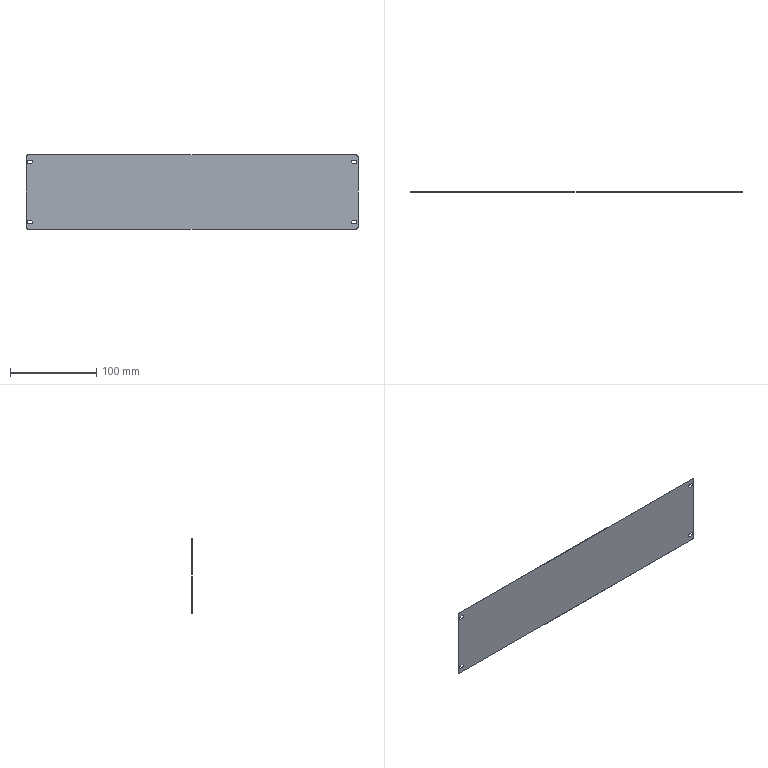Part | STEP file | LES120 steel strip^FTH120-PD-direct-drive motor | 1 solid | 26 faces | box 385.8 x 0.15 x 86 mm | volume 4964 mm3 | plane 14 | cylinder 12 | commonest cylinder face diameters 4 x12
STEP:
#1=CARTESIAN_POINT('',(190.9,0.15,-43.));
#2=VERTEX_POINT('',#1);
#3=CARTESIAN_POINT('',(192.9,0.15,-41.));
#4=VERTEX_POINT('',#3);
#5=CARTESIAN_POINT('',(190.9,0.15,-41.));
#6=DIRECTION('',(0.,-1.,0.));
#7=DIRECTION('',(0.,0.,-1.));
#8=AXIS2_PLACEMENT_3D('',#5,#6,#7);
#9=CIRCLE('',#8,2.);
#10=EDGE_CURVE('',#2,#4,#9,.T.);
#11=ORIENTED_EDGE('',*,*,#10,.F.);
#12=CARTESIAN_POINT('',(-190.9,0.15,-43.));
#13=VERTEX_POINT('',#12);
#14=CARTESIAN_POINT('',(0.,0.15,-43.));
#15=DIRECTION('',(1.,0.,0.));
#16=VECTOR('',#15,1000.);
#17=LINE('',#14,#16);
#18=EDGE_CURVE('',#13,#2,#17,.T.);
#19=ORIENTED_EDGE('',*,*,#18,.F.);
#20=CARTESIAN_POINT('',(-192.9,0.15,-41.));
#21=VERTEX_POINT('',#20);
#22=CARTESIAN_POINT('',(-190.9,0.15,-41.));
#23=DIRECTION('',(0.,-1.,0.));
#24=DIRECTION('',(0.,0.,-1.));
#25=AXIS2_PLACEMENT_3D('',#22,#23,#24);
#26=CIRCLE('',#25,2.);
#27=EDGE_CURVE('',#21,#13,#26,.T.);
#28=ORIENTED_EDGE('',*,*,#27,.F.);
#29=CARTESIAN_POINT('',(-192.9,0.15,41.));
#30=VERTEX_POINT('',#29);
#31=CARTESIAN_POINT('',(-192.9,0.15,0.));
#32=DIRECTION('',(0.,0.,-1.));
#33=VECTOR('',#32,1000.);
#34=LINE('',#31,#33);
#35=EDGE_CURVE('',#30,#21,#34,.T.);
#36=ORIENTED_EDGE('',*,*,#35,.F.);
#37=CARTESIAN_POINT('',(-190.9,0.15,43.));
#38=VERTEX_POINT('',#37);
#39=CARTESIAN_POINT('',(-190.9,0.15,41.));
#40=DIRECTION('',(0.,-1.,0.));
#41=DIRECTION('',(0.,0.,-1.));
#42=AXIS2_PLACEMENT_3D('',#39,#40,#41);
#43=CIRCLE('',#42,2.);
#44=EDGE_CURVE('',#38,#30,#43,.T.);
#45=ORIENTED_EDGE('',*,*,#44,.F.);
#46=CARTESIAN_POINT('',(190.9,0.15,43.));
#47=VERTEX_POINT('',#46);
#48=CARTESIAN_POINT('',(0.,0.15,43.));
#49=DIRECTION('',(-1.,0.,0.));
#50=VECTOR('',#49,1000.);
#51=LINE('',#48,#50);
#52=EDGE_CURVE('',#47,#38,#51,.T.);
#53=ORIENTED_EDGE('',*,*,#52,.F.);
#54=CARTESIAN_POINT('',(192.9,0.15,41.));
#55=VERTEX_POINT('',#54);
#56=CARTESIAN_POINT('',(190.9,0.15,41.));
#57=DIRECTION('',(0.,-1.,0.));
#58=DIRECTION('',(0.,0.,-1.));
#59=AXIS2_PLACEMENT_3D('',#56,#57,#58);
#60=CIRCLE('',#59,2.);
#61=EDGE_CURVE('',#55,#47,#60,.T.);
#62=ORIENTED_EDGE('',*,*,#61,.F.);
#63=CARTESIAN_POINT('',(192.9,0.15,0.));
#64=DIRECTION('',(0.,0.,1.));
#65=VECTOR('',#64,1000.);
#66=LINE('',#63,#65);
#67=EDGE_CURVE('',#4,#55,#66,.T.);
#68=ORIENTED_EDGE('',*,*,#67,.F.);
#69=EDGE_LOOP('',(#11,#19,#28,#36,#45,#53,#62,#68));
#70=FACE_OUTER_BOUND('',#69,.T.);
#71=CARTESIAN_POINT('',(-187.4,0.15,-32.9));
#72=VERTEX_POINT('',#71);
#73=CARTESIAN_POINT('',(-187.4,0.15,-36.9));
#74=VERTEX_POINT('',#73);
#75=CARTESIAN_POINT('',(-187.4,0.15,-34.9));
#76=DIRECTION('',(0.,1.,0.));
#77=DIRECTION('',(0.,0.,1.));
#78=AXIS2_PLACEMENT_3D('',#75,#76,#77);
#79=CIRCLE('',#78,2.);
#80=EDGE_CURVE('',#72,#74,#79,.T.);
#81=ORIENTED_EDGE('',*,*,#80,.F.);
#82=CARTESIAN_POINT('',(-189.4,0.15,-32.9));
#83=VERTEX_POINT('',#82);
#84=CARTESIAN_POINT('',(0.,0.15,-32.9));
#85=DIRECTION('',(1.,0.,0.));
#86=VECTOR('',#85,1000.);
#87=LINE('',#84,#86);
#88=EDGE_CURVE('',#83,#72,#87,.T.);
#89=ORIENTED_EDGE('',*,*,#88,.F.);
#90=CARTESIAN_POINT('',(-189.4,0.15,-36.9));
#91=VERTEX_POINT('',#90);
#92=CARTESIAN_POINT('',(-189.4,0.15,-34.9));
#93=DIRECTION('',(0.,1.,0.));
#94=DIRECTION('',(0.,0.,1.));
#95=AXIS2_PLACEMENT_3D('',#92,#93,#94);
#96=CIRCLE('',#95,2.);
#97=EDGE_CURVE('',#91,#83,#96,.T.);
#98=ORIENTED_EDGE('',*,*,#97,.F.);
#99=CARTESIAN_POINT('',(0.,0.15,-36.9));
#100=DIRECTION('',(-1.,0.,0.));
#101=VECTOR('',#100,1000.);
#102=LINE('',#99,#101);
#103=EDGE_CURVE('',#74,#91,#102,.T.);
#104=ORIENTED_EDGE('',*,*,#103,.F.);
#105=EDGE_LOOP('',(#81,#89,#98,#104));
#106=FACE_BOUND('',#105,.T.);
#107=CARTESIAN_POINT('',(-189.4,0.15,32.9));
#108=VERTEX_POINT('',#107);
#109=CARTESIAN_POINT('',(-189.4,0.15,36.9));
#110=VERTEX_POINT('',#109);
#111=CARTESIAN_POINT('',(-189.4,0.15,34.9));
#112=DIRECTION('',(0.,1.,0.));
#113=DIRECTION('',(0.,0.,1.));
#114=AXIS2_PLACEMENT_3D('',#111,#112,#113);
#115=CIRCLE('',#114,2.);
#116=EDGE_CURVE('',#108,#110,#115,.T.);
#117=ORIENTED_EDGE('',*,*,#116,.F.);
#118=CARTESIAN_POINT('',(-187.4,0.15,32.9));
#119=VERTEX_POINT('',#118);
#120=CARTESIAN_POINT('',(0.,0.15,32.9));
#121=DIRECTION('',(-1.,0.,0.));
#122=VECTOR('',#121,1000.);
#123=LINE('',#120,#122);
#124=EDGE_CURVE('',#119,#108,#123,.T.);
#125=ORIENTED_EDGE('',*,*,#124,.F.);
#126=CARTESIAN_POINT('',(-187.4,0.15,36.9));
#127=VERTEX_POINT('',#126);
#128=CARTESIAN_POINT('',(-187.4,0.15,34.9));
#129=DIRECTION('',(0.,1.,0.));
#130=DIRECTION('',(0.,0.,1.));
#131=AXIS2_PLACEMENT_3D('',#128,#129,#130);
#132=CIRCLE('',#131,2.);
#133=EDGE_CURVE('',#127,#119,#132,.T.);
#134=ORIENTED_EDGE('',*,*,#133,.F.);
#135=CARTESIAN_POINT('',(0.,0.15,36.9));
#136=DIRECTION('',(1.,0.,0.));
#137=VECTOR('',#136,1000.);
#138=LINE('',#135,#137);
#139=EDGE_CURVE('',#110,#127,#138,.T.);
#140=ORIENTED_EDGE('',*,*,#139,.F.);
#141=EDGE_LOOP('',(#117,#125,#134,#140));
#142=FACE_BOUND('',#141,.T.);
#143=CARTESIAN_POINT('',(189.4,0.15,36.9));
#144=VERTEX_POINT('',#143);
#145=CARTESIAN_POINT('',(189.4,0.15,32.9));
#146=VERTEX_POINT('',#145);
#147=CARTESIAN_POINT('',(189.4,0.15,34.9));
#148=DIRECTION('',(0.,1.,0.));
#149=DIRECTION('',(0.,0.,1.));
#150=AXIS2_PLACEMENT_3D('',#147,#148,#149);
#151=CIRCLE('',#150,2.);
#152=EDGE_CURVE('',#144,#146,#151,.T.);
#153=ORIENTED_EDGE('',*,*,#152,.F.);
#154=CARTESIAN_POINT('',(187.4,0.15,36.9));
#155=VERTEX_POINT('',#154);
#156=CARTESIAN_POINT('',(0.,0.15,36.9));
#157=DIRECTION('',(1.,0.,0.));
#158=VECTOR('',#157,1000.);
#159=LINE('',#156,#158);
#160=EDGE_CURVE('',#155,#144,#159,.T.);
#161=ORIENTED_EDGE('',*,*,#160,.F.);
#162=CARTESIAN_POINT('',(187.4,0.15,32.9));
#163=VERTEX_POINT('',#162);
#164=CARTESIAN_POINT('',(187.4,0.15,34.9));
#165=DIRECTION('',(0.,1.,0.));
#166=DIRECTION('',(0.,0.,1.));
#167=AXIS2_PLACEMENT_3D('',#164,#165,#166);
#168=CIRCLE('',#167,2.);
#169=EDGE_CURVE('',#163,#155,#168,.T.);
#170=ORIENTED_EDGE('',*,*,#169,.F.);
#171=CARTESIAN_POINT('',(0.,0.15,32.9));
#172=DIRECTION('',(-1.,0.,0.));
#173=VECTOR('',#172,1000.);
#174=LINE('',#171,#173);
#175=EDGE_CURVE('',#146,#163,#174,.T.);
#176=ORIENTED_EDGE('',*,*,#175,.F.);
#177=EDGE_LOOP('',(#153,#161,#170,#176));
#178=FACE_BOUND('',#177,.T.);
#179=CARTESIAN_POINT('',(189.4,0.15,-32.9));
#180=VERTEX_POINT('',#179);
#181=CARTESIAN_POINT('',(189.4,0.15,-36.9));
#182=VERTEX_POINT('',#181);
#183=CARTESIAN_POINT('',(189.4,0.15,-34.9));
#184=DIRECTION('',(0.,1.,0.));
#185=DIRECTION('',(0.,0.,1.));
#186=AXIS2_PLACEMENT_3D('',#183,#184,#185);
#187=CIRCLE('',#186,2.);
#188=EDGE_CURVE('',#180,#182,#187,.T.);
#189=ORIENTED_EDGE('',*,*,#188,.F.);
#190=CARTESIAN_POINT('',(187.4,0.15,-32.9));
#191=VERTEX_POINT('',#190);
#192=CARTESIAN_POINT('',(0.,0.15,-32.9));
#193=DIRECTION('',(1.,0.,0.));
#194=VECTOR('',#193,1000.);
#195=LINE('',#192,#194);
#196=EDGE_CURVE('',#191,#180,#195,.T.);
#197=ORIENTED_EDGE('',*,*,#196,.F.);
#198=CARTESIAN_POINT('',(187.4,0.15,-36.9));
#199=VERTEX_POINT('',#198);
#200=CARTESIAN_POINT('',(187.4,0.15,-34.9));
#201=DIRECTION('',(0.,1.,0.));
#202=DIRECTION('',(0.,0.,1.));
#203=AXIS2_PLACEMENT_3D('',#200,#201,#202);
#204=CIRCLE('',#203,2.);
#205=EDGE_CURVE('',#199,#191,#204,.T.);
#206=ORIENTED_EDGE('',*,*,#205,.F.);
#207=CARTESIAN_POINT('',(0.,0.15,-36.9));
#208=DIRECTION('',(-1.,0.,0.));
#209=VECTOR('',#208,1000.);
#210=LINE('',#207,#209);
#211=EDGE_CURVE('',#182,#199,#210,.T.);
#212=ORIENTED_EDGE('',*,*,#211,.F.);
#213=EDGE_LOOP('',(#189,#197,#206,#212));
#214=FACE_BOUND('',#213,.T.);
#215=CARTESIAN_POINT('',(0.,0.15,0.));
#216=DIRECTION('',(0.,-1.,0.));
#217=DIRECTION('',(0.,0.,-1.));
#218=AXIS2_PLACEMENT_3D('',#215,#216,#217);
#219=PLANE('',#218);
#220=ADVANCED_FACE('',(#70,#106,#142,#178,#214),#219,.F.);
#221=CARTESIAN_POINT('',(192.9,0.,-41.));
#222=VERTEX_POINT('',#221);
#223=CARTESIAN_POINT('',(192.9,0.15,-41.));
#224=DIRECTION('',(0.,-1.,0.));
#225=VECTOR('',#224,1000.);
#226=LINE('',#223,#225);
#227=EDGE_CURVE('',#4,#222,#226,.T.);
#228=ORIENTED_EDGE('',*,*,#227,.F.);
#229=ORIENTED_EDGE('',*,*,#67,.T.);
#230=CARTESIAN_POINT('',(192.9,0.,41.));
#231=VERTEX_POINT('',#230);
#232=CARTESIAN_POINT('',(192.9,0.15,41.));
#233=DIRECTION('',(0.,1.,0.));
#234=VECTOR('',#233,1000.);
#235=LINE('',#232,#234);
#236=EDGE_CURVE('',#231,#55,#235,.T.);
#237=ORIENTED_EDGE('',*,*,#236,.F.);
#238=CARTESIAN_POINT('',(192.9,0.,43.));
#239=DIRECTION('',(0.,0.,1.));
#240=VECTOR('',#239,1000.);
#241=LINE('',#238,#240);
#242=EDGE_CURVE('',#222,#231,#241,.T.);
#243=ORIENTED_EDGE('',*,*,#242,.F.);
#244=EDGE_LOOP('',(#228,#229,#237,#243));
#245=FACE_OUTER_BOUND('',#244,.T.);
#246=CARTESIAN_POINT('',(192.9,0.15,43.));
#247=DIRECTION('',(-1.,0.,0.));
#248=DIRECTION('',(0.,0.,1.));
#249=AXIS2_PLACEMENT_3D('',#246,#247,#248);
#250=PLANE('',#249);
#251=ADVANCED_FACE('',(#245),#250,.F.);
#252=CARTESIAN_POINT('',(190.9,0.,-43.));
#253=VERTEX_POINT('',#252);
#254=CARTESIAN_POINT('',(190.9,0.,-41.));
#255=DIRECTION('',(0.,1.,0.));
#256=DIRECTION('',(0.,0.,-1.));
#257=AXIS2_PLACEMENT_3D('',#254,#255,#256);
#258=CIRCLE('',#257,2.);
#259=EDGE_CURVE('',#222,#253,#258,.T.);
#260=ORIENTED_EDGE('',*,*,#259,.T.);
#261=CARTESIAN_POINT('',(190.9,0.15,-43.));
#262=DIRECTION('',(0.,1.,0.));
#263=VECTOR('',#262,1000.);
#264=LINE('',#261,#263);
#265=EDGE_CURVE('',#253,#2,#264,.T.);
#266=ORIENTED_EDGE('',*,*,#265,.T.);
#267=ORIENTED_EDGE('',*,*,#10,.T.);
#268=ORIENTED_EDGE('',*,*,#227,.T.);
#269=EDGE_LOOP('',(#260,#266,#267,#268));
#270=FACE_OUTER_BOUND('',#269,.T.);
#271=CARTESIAN_POINT('',(190.9,0.15,-41.));
#272=DIRECTION('',(0.,-1.,0.));
#273=DIRECTION('',(0.,0.,-1.));
#274=AXIS2_PLACEMENT_3D('',#271,#272,#273);
#275=CYLINDRICAL_SURFACE('',#274,2.);
#276=ADVANCED_FACE('',(#270),#275,.T.);
#277=ORIENTED_EDGE('',*,*,#265,.F.);
#278=CARTESIAN_POINT('',(-190.9,0.,-43.));
#279=VERTEX_POINT('',#278);
#280=CARTESIAN_POINT('',(-192.9,0.,-43.));
#281=DIRECTION('',(1.,0.,0.));
#282=VECTOR('',#281,1000.);
#283=LINE('',#280,#282);
#284=EDGE_CURVE('',#279,#253,#283,.T.);
#285=ORIENTED_EDGE('',*,*,#284,.F.);
#286=CARTESIAN_POINT('',(-190.9,0.15,-43.));
#287=DIRECTION('',(0.,-1.,0.));
#288=VECTOR('',#287,1000.);
#289=LINE('',#286,#288);
#290=EDGE_CURVE('',#13,#279,#289,.T.);
#291=ORIENTED_EDGE('',*,*,#290,.F.);
#292=ORIENTED_EDGE('',*,*,#18,.T.);
#293=EDGE_LOOP('',(#277,#285,#291,#292));
#294=FACE_OUTER_BOUND('',#293,.T.);
#295=CARTESIAN_POINT('',(-192.9,0.15,-43.));
#296=DIRECTION('',(0.,0.,1.));
#297=DIRECTION('',(1.,0.,0.));
#298=AXIS2_PLACEMENT_3D('',#295,#296,#297);
#299=PLANE('',#298);
#300=ADVANCED_FACE('',(#294),#299,.F.);
#301=CARTESIAN_POINT('',(-192.9,0.,-41.));
#302=VERTEX_POINT('',#301);
#303=CARTESIAN_POINT('',(-190.9,0.,-41.));
#304=DIRECTION('',(0.,1.,0.));
#305=DIRECTION('',(0.,0.,-1.));
#306=AXIS2_PLACEMENT_3D('',#303,#304,#305);
#307=CIRCLE('',#306,2.);
#308=EDGE_CURVE('',#279,#302,#307,.T.);
#309=ORIENTED_EDGE('',*,*,#308,.T.);
#310=CARTESIAN_POINT('',(-192.9,0.15,-41.));
#311=DIRECTION('',(0.,1.,0.));
#312=VECTOR('',#311,1000.);
#313=LINE('',#310,#312);
#314=EDGE_CURVE('',#302,#21,#313,.T.);
#315=ORIENTED_EDGE('',*,*,#314,.T.);
#316=ORIENTED_EDGE('',*,*,#27,.T.);
#317=ORIENTED_EDGE('',*,*,#290,.T.);
#318=EDGE_LOOP('',(#309,#315,#316,#317));
#319=FACE_OUTER_BOUND('',#318,.T.);
#320=CARTESIAN_POINT('',(-190.9,0.15,-41.));
#321=DIRECTION('',(0.,-1.,0.));
#322=DIRECTION('',(0.,0.,-1.));
#323=AXIS2_PLACEMENT_3D('',#320,#321,#322);
#324=CYLINDRICAL_SURFACE('',#323,2.);
#325=ADVANCED_FACE('',(#319),#324,.T.);
#326=ORIENTED_EDGE('',*,*,#314,.F.);
#327=CARTESIAN_POINT('',(-192.9,0.,41.));
#328=VERTEX_POINT('',#327);
#329=CARTESIAN_POINT('',(-192.9,0.,43.));
#330=DIRECTION('',(0.,0.,-1.));
#331=VECTOR('',#330,1000.);
#332=LINE('',#329,#331);
#333=EDGE_CURVE('',#328,#302,#332,.T.);
#334=ORIENTED_EDGE('',*,*,#333,.F.);
#335=CARTESIAN_POINT('',(-192.9,0.15,41.));
#336=DIRECTION('',(0.,-1.,0.));
#337=VECTOR('',#336,1000.);
#338=LINE('',#335,#337);
#339=EDGE_CURVE('',#30,#328,#338,.T.);
#340=ORIENTED_EDGE('',*,*,#339,.F.);
#341=ORIENTED_EDGE('',*,*,#35,.T.);
#342=EDGE_LOOP('',(#326,#334,#340,#341));
#343=FACE_OUTER_BOUND('',#342,.T.);
#344=CARTESIAN_POINT('',(-192.9,0.15,43.));
#345=DIRECTION('',(1.,0.,0.));
#346=DIRECTION('',(0.,0.,-1.));
#347=AXIS2_PLACEMENT_3D('',#344,#345,#346);
#348=PLANE('',#347);
#349=ADVANCED_FACE('',(#343),#348,.F.);
#350=CARTESIAN_POINT('',(-190.9,0.,43.));
#351=VERTEX_POINT('',#350);
#352=CARTESIAN_POINT('',(-190.9,0.,41.));
#353=DIRECTION('',(0.,1.,0.));
#354=DIRECTION('',(0.,0.,-1.));
#355=AXIS2_PLACEMENT_3D('',#352,#353,#354);
#356=CIRCLE('',#355,2.);
#357=EDGE_CURVE('',#328,#351,#356,.T.);
#358=ORIENTED_EDGE('',*,*,#357,.T.);
#359=CARTESIAN_POINT('',(-190.9,0.15,43.));
#360=DIRECTION('',(0.,1.,0.));
#361=VECTOR('',#360,1000.);
#362=LINE('',#359,#361);
#363=EDGE_CURVE('',#351,#38,#362,.T.);
#364=ORIENTED_EDGE('',*,*,#363,.T.);
#365=ORIENTED_EDGE('',*,*,#44,.T.);
#366=ORIENTED_EDGE('',*,*,#339,.T.);
#367=EDGE_LOOP('',(#358,#364,#365,#366));
#368=FACE_OUTER_BOUND('',#367,.T.);
#369=CARTESIAN_POINT('',(-190.9,0.15,41.));
#370=DIRECTION('',(0.,-1.,0.));
#371=DIRECTION('',(0.,0.,-1.));
#372=AXIS2_PLACEMENT_3D('',#369,#370,#371);
#373=CYLINDRICAL_SURFACE('',#372,2.);
#374=ADVANCED_FACE('',(#368),#373,.T.);
#375=CARTESIAN_POINT('',(190.9,0.,43.));
#376=VERTEX_POINT('',#375);
#377=CARTESIAN_POINT('',(190.9,0.15,43.));
#378=DIRECTION('',(0.,-1.,0.));
#379=VECTOR('',#378,1000.);
#380=LINE('',#377,#379);
#381=EDGE_CURVE('',#47,#376,#380,.T.);
#382=ORIENTED_EDGE('',*,*,#381,.F.);
#383=ORIENTED_EDGE('',*,*,#52,.T.);
#384=ORIENTED_EDGE('',*,*,#363,.F.);
#385=CARTESIAN_POINT('',(-192.9,0.,43.));
#386=DIRECTION('',(-1.,0.,0.));
#387=VECTOR('',#386,1000.);
#388=LINE('',#385,#387);
#389=EDGE_CURVE('',#376,#351,#388,.T.);
#390=ORIENTED_EDGE('',*,*,#389,.F.);
#391=EDGE_LOOP('',(#382,#383,#384,#390));
#392=FACE_OUTER_BOUND('',#391,.T.);
#393=CARTESIAN_POINT('',(-192.9,0.15,43.));
#394=DIRECTION('',(0.,0.,-1.));
#395=DIRECTION('',(-1.,0.,0.));
#396=AXIS2_PLACEMENT_3D('',#393,#394,#395);
#397=PLANE('',#396);
#398=ADVANCED_FACE('',(#392),#397,.F.);
#399=CARTESIAN_POINT('',(190.9,0.,41.));
#400=DIRECTION('',(0.,1.,0.));
#401=DIRECTION('',(0.,0.,-1.));
#402=AXIS2_PLACEMENT_3D('',#399,#400,#401);
#403=CIRCLE('',#402,2.);
#404=EDGE_CURVE('',#376,#231,#403,.T.);
#405=ORIENTED_EDGE('',*,*,#404,.T.);
#406=ORIENTED_EDGE('',*,*,#236,.T.);
#407=ORIENTED_EDGE('',*,*,#61,.T.);
#408=ORIENTED_EDGE('',*,*,#381,.T.);
#409=EDGE_LOOP('',(#405,#406,#407,#408));
#410=FACE_OUTER_BOUND('',#409,.T.);
#411=CARTESIAN_POINT('',(190.9,0.15,41.));
#412=DIRECTION('',(0.,-1.,0.));
#413=DIRECTION('',(0.,0.,-1.));
#414=AXIS2_PLACEMENT_3D('',#411,#412,#413);
#415=CYLINDRICAL_SURFACE('',#414,2.);
#416=ADVANCED_FACE('',(#410),#415,.T.);
#417=CARTESIAN_POINT('',(-189.4,0.,-36.9));
#418=VERTEX_POINT('',#417);
#419=CARTESIAN_POINT('',(-189.4,0.,-36.9));
#420=DIRECTION('',(0.,1.,0.));
#421=VECTOR('',#420,1000.);
#422=LINE('',#419,#421);
#423=EDGE_CURVE('',#418,#91,#422,.T.);
#424=ORIENTED_EDGE('',*,*,#423,.F.);
#425=CARTESIAN_POINT('',(-187.4,0.,-36.9));
#426=VERTEX_POINT('',#425);
#427=CARTESIAN_POINT('',(-189.4,0.,-36.9));
#428=DIRECTION('',(-1.,0.,0.));
#429=VECTOR('',#428,1000.);
#430=LINE('',#427,#429);
#431=EDGE_CURVE('',#426,#418,#430,.T.);
#432=ORIENTED_EDGE('',*,*,#431,.F.);
#433=CARTESIAN_POINT('',(-187.4,0.,-36.9));
#434=DIRECTION('',(0.,-1.,0.));
#435=VECTOR('',#434,1000.);
#436=LINE('',#433,#435);
#437=EDGE_CURVE('',#74,#426,#436,.T.);
#438=ORIENTED_EDGE('',*,*,#437,.F.);
#439=ORIENTED_EDGE('',*,*,#103,.T.);
#440=EDGE_LOOP('',(#424,#432,#438,#439));
#441=FACE_OUTER_BOUND('',#440,.T.);
#442=CARTESIAN_POINT('',(-189.4,0.,-36.9));
#443=DIRECTION('',(0.,0.,-1.));
#444=DIRECTION('',(-1.,0.,0.));
#445=AXIS2_PLACEMENT_3D('',#442,#443,#444);
#446=PLANE('',#445);
#447=ADVANCED_FACE('',(#441),#446,.F.);
#448=ORIENTED_EDGE('',*,*,#437,.T.);
#449=CARTESIAN_POINT('',(-187.4,0.,-32.9));
#450=VERTEX_POINT('',#449);
#451=CARTESIAN_POINT('',(-187.4,0.,-34.9));
#452=DIRECTION('',(0.,1.,0.));
#453=DIRECTION('',(0.,0.,1.));
#454=AXIS2_PLACEMENT_3D('',#451,#452,#453);
#455=CIRCLE('',#454,2.);
#456=EDGE_CURVE('',#450,#426,#455,.T.);
#457=ORIENTED_EDGE('',*,*,#456,.F.);
#458=CARTESIAN_POINT('',(-187.4,0.,-32.9));
#459=DIRECTION('',(0.,-1.,0.));
#460=VECTOR('',#459,1000.);
#461=LINE('',#458,#460);
#462=EDGE_CURVE('',#72,#450,#461,.T.);
#463=ORIENTED_EDGE('',*,*,#462,.F.);
#464=ORIENTED_EDGE('',*,*,#80,.T.);
#465=EDGE_LOOP('',(#448,#457,#463,#464));
#466=FACE_OUTER_BOUND('',#465,.T.);
#467=CARTESIAN_POINT('',(-187.4,0.,-34.9));
#468=DIRECTION('',(0.,1.,0.));
#469=DIRECTION('',(0.,0.,1.));
#470=AXIS2_PLACEMENT_3D('',#467,#468,#469);
#471=CYLINDRICAL_SURFACE('',#470,2.);
#472=ADVANCED_FACE('',(#466),#471,.F.);
#473=ORIENTED_EDGE('',*,*,#462,.T.);
#474=CARTESIAN_POINT('',(-189.4,0.,-32.9));
#475=VERTEX_POINT('',#474);
#476=CARTESIAN_POINT('',(-189.4,0.,-32.9));
#477=DIRECTION('',(1.,0.,0.));
#478=VECTOR('',#477,1000.);
#479=LINE('',#476,#478);
#480=EDGE_CURVE('',#475,#450,#479,.T.);
#481=ORIENTED_EDGE('',*,*,#480,.F.);
#482=CARTESIAN_POINT('',(-189.4,0.,-32.9));
#483=DIRECTION('',(0.,-1.,0.));
#484=VECTOR('',#483,1000.);
#485=LINE('',#482,#484);
#486=EDGE_CURVE('',#83,#475,#485,.T.);
#487=ORIENTED_EDGE('',*,*,#486,.F.);
#488=ORIENTED_EDGE('',*,*,#88,.T.);
#489=EDGE_LOOP('',(#473,#481,#487,#488));
#490=FACE_OUTER_BOUND('',#489,.T.);
#491=CARTESIAN_POINT('',(-189.4,0.,-32.9));
#492=DIRECTION('',(0.,0.,1.));
#493=DIRECTION('',(1.,0.,0.));
#494=AXIS2_PLACEMENT_3D('',#491,#492,#493);
#495=PLANE('',#494);
#496=ADVANCED_FACE('',(#490),#495,.F.);
#497=ORIENTED_EDGE('',*,*,#486,.T.);
#498=CARTESIAN_POINT('',(-189.4,0.,-34.9));
#499=DIRECTION('',(0.,1.,0.));
#500=DIRECTION('',(0.,0.,1.));
#501=AXIS2_PLACEMENT_3D('',#498,#499,#500);
#502=CIRCLE('',#501,2.);
#503=EDGE_CURVE('',#418,#475,#502,.T.);
#504=ORIENTED_EDGE('',*,*,#503,.F.);
#505=ORIENTED_EDGE('',*,*,#423,.T.);
#506=ORIENTED_EDGE('',*,*,#97,.T.);
#507=EDGE_LOOP('',(#497,#504,#505,#506));
#508=FACE_OUTER_BOUND('',#507,.T.);
#509=CARTESIAN_POINT('',(-189.4,0.,-34.9));
#510=DIRECTION('',(0.,1.,0.));
#511=DIRECTION('',(0.,0.,1.));
#512=AXIS2_PLACEMENT_3D('',#509,#510,#511);
#513=CYLINDRICAL_SURFACE('',#512,2.);
#514=ADVANCED_FACE('',(#508),#513,.F.);
#515=CARTESIAN_POINT('',(-187.4,0.,36.9));
#516=VERTEX_POINT('',#515);
#517=CARTESIAN_POINT('',(-187.4,0.,36.9));
#518=DIRECTION('',(0.,1.,0.));
#519=VECTOR('',#518,1000.);
#520=LINE('',#517,#519);
#521=EDGE_CURVE('',#516,#127,#520,.T.);
#522=ORIENTED_EDGE('',*,*,#521,.F.);
#523=CARTESIAN_POINT('',(-189.4,0.,36.9));
#524=VERTEX_POINT('',#523);
#525=CARTESIAN_POINT('',(-189.4,0.,36.9));
#526=DIRECTION('',(1.,0.,0.));
#527=VECTOR('',#526,1000.);
#528=LINE('',#525,#527);
#529=EDGE_CURVE('',#524,#516,#528,.T.);
#530=ORIENTED_EDGE('',*,*,#529,.F.);
#531=CARTESIAN_POINT('',(-189.4,0.,36.9));
#532=DIRECTION('',(0.,-1.,0.));
#533=VECTOR('',#532,1000.);
#534=LINE('',#531,#533);
#535=EDGE_CURVE('',#110,#524,#534,.T.);
#536=ORIENTED_EDGE('',*,*,#535,.F.);
#537=ORIENTED_EDGE('',*,*,#139,.T.);
#538=EDGE_LOOP('',(#522,#530,#536,#537));
#539=FACE_OUTER_BOUND('',#538,.T.);
#540=CARTESIAN_POINT('',(-189.4,0.,36.9));
#541=DIRECTION('',(0.,0.,1.));
#542=DIRECTION('',(1.,0.,0.));
#543=AXIS2_PLACEMENT_3D('',#540,#541,#542);
#544=PLANE('',#543);
#545=ADVANCED_FACE('',(#539),#544,.F.);
#546=ORIENTED_EDGE('',*,*,#535,.T.);
#547=CARTESIAN_POINT('',(-189.4,0.,32.9));
#548=VERTEX_POINT('',#547);
#549=CARTESIAN_POINT('',(-189.4,0.,34.9));
#550=DIRECTION('',(0.,1.,0.));
#551=DIRECTION('',(0.,0.,1.));
#552=AXIS2_PLACEMENT_3D('',#549,#550,#551);
#553=CIRCLE('',#552,2.);
#554=EDGE_CURVE('',#548,#524,#553,.T.);
#555=ORIENTED_EDGE('',*,*,#554,.F.);
#556=CARTESIAN_POINT('',(-189.4,0.,32.9));
#557=DIRECTION('',(0.,-1.,0.));
#558=VECTOR('',#557,1000.);
#559=LINE('',#556,#558);
#560=EDGE_CURVE('',#108,#548,#559,.T.);
#561=ORIENTED_EDGE('',*,*,#560,.F.);
#562=ORIENTED_EDGE('',*,*,#116,.T.);
#563=EDGE_LOOP('',(#546,#555,#561,#562));
#564=FACE_OUTER_BOUND('',#563,.T.);
#565=CARTESIAN_POINT('',(-189.4,0.,34.9));
#566=DIRECTION('',(0.,1.,0.));
#567=DIRECTION('',(0.,0.,1.));
#568=AXIS2_PLACEMENT_3D('',#565,#566,#567);
#569=CYLINDRICAL_SURFACE('',#568,2.);
#570=ADVANCED_FACE('',(#564),#569,.F.);
#571=ORIENTED_EDGE('',*,*,#560,.T.);
#572=CARTESIAN_POINT('',(-187.4,0.,32.9));
#573=VERTEX_POINT('',#572);
#574=CARTESIAN_POINT('',(-189.4,0.,32.9));
#575=DIRECTION('',(-1.,0.,0.));
#576=VECTOR('',#575,1000.);
#577=LINE('',#574,#576);
#578=EDGE_CURVE('',#573,#548,#577,.T.);
#579=ORIENTED_EDGE('',*,*,#578,.F.);
#580=CARTESIAN_POINT('',(-187.4,0.,32.9));
#581=DIRECTION('',(0.,-1.,0.));
#582=VECTOR('',#581,1000.);
#583=LINE('',#580,#582);
#584=EDGE_CURVE('',#119,#573,#583,.T.);
#585=ORIENTED_EDGE('',*,*,#584,.F.);
#586=ORIENTED_EDGE('',*,*,#124,.T.);
#587=EDGE_LOOP('',(#571,#579,#585,#586));
#588=FACE_OUTER_BOUND('',#587,.T.);
#589=CARTESIAN_POINT('',(-189.4,0.,32.9));
#590=DIRECTION('',(0.,0.,-1.));
#591=DIRECTION('',(-1.,0.,0.));
#592=AXIS2_PLACEMENT_3D('',#589,#590,#591);
#593=PLANE('',#592);
#594=ADVANCED_FACE('',(#588),#593,.F.);
#595=ORIENTED_EDGE('',*,*,#584,.T.);
#596=CARTESIAN_POINT('',(-187.4,0.,34.9));
#597=DIRECTION('',(0.,1.,0.));
#598=DIRECTION('',(0.,0.,1.));
#599=AXIS2_PLACEMENT_3D('',#596,#597,#598);
#600=CIRCLE('',#599,2.);
#601=EDGE_CURVE('',#516,#573,#600,.T.);
#602=ORIENTED_EDGE('',*,*,#601,.F.);
#603=ORIENTED_EDGE('',*,*,#521,.T.);
#604=ORIENTED_EDGE('',*,*,#133,.T.);
#605=EDGE_LOOP('',(#595,#602,#603,#604));
#606=FACE_OUTER_BOUND('',#605,.T.);
#607=CARTESIAN_POINT('',(-187.4,0.,34.9));
#608=DIRECTION('',(0.,1.,0.));
#609=DIRECTION('',(0.,0.,1.));
#610=AXIS2_PLACEMENT_3D('',#607,#608,#609);
#611=CYLINDRICAL_SURFACE('',#610,2.);
#612=ADVANCED_FACE('',(#606),#611,.F.);
#613=CARTESIAN_POINT('',(187.4,0.,32.9));
#614=VERTEX_POINT('',#613);
#615=CARTESIAN_POINT('',(187.4,0.,32.9));
#616=DIRECTION('',(0.,1.,0.));
#617=VECTOR('',#616,1000.);
#618=LINE('',#615,#617);
#619=EDGE_CURVE('',#614,#163,#618,.T.);
#620=ORIENTED_EDGE('',*,*,#619,.F.);
#621=CARTESIAN_POINT('',(189.4,0.,32.9));
#622=VERTEX_POINT('',#621);
#623=CARTESIAN_POINT('',(189.4,0.,32.9));
#624=DIRECTION('',(-1.,0.,0.));
#625=VECTOR('',#624,1000.);
#626=LINE('',#623,#625);
#627=EDGE_CURVE('',#622,#614,#626,.T.);
#628=ORIENTED_EDGE('',*,*,#627,.F.);
#629=CARTESIAN_POINT('',(189.4,0.,32.9));
#630=DIRECTION('',(0.,-1.,0.));
#631=VECTOR('',#630,1000.);
#632=LINE('',#629,#631);
#633=EDGE_CURVE('',#146,#622,#632,.T.);
#634=ORIENTED_EDGE('',*,*,#633,.F.);
#635=ORIENTED_EDGE('',*,*,#175,.T.);
#636=EDGE_LOOP('',(#620,#628,#634,#635));
#637=FACE_OUTER_BOUND('',#636,.T.);
#638=CARTESIAN_POINT('',(189.4,0.,32.9));
#639=DIRECTION('',(0.,0.,-1.));
#640=DIRECTION('',(-1.,0.,0.));
#641=AXIS2_PLACEMENT_3D('',#638,#639,#640);
#642=PLANE('',#641);
#643=ADVANCED_FACE('',(#637),#642,.F.);
#644=ORIENTED_EDGE('',*,*,#633,.T.);
#645=CARTESIAN_POINT('',(189.4,0.,36.9));
#646=VERTEX_POINT('',#645);
#647=CARTESIAN_POINT('',(189.4,0.,34.9));
#648=DIRECTION('',(0.,1.,0.));
#649=DIRECTION('',(0.,0.,1.));
#650=AXIS2_PLACEMENT_3D('',#647,#648,#649);
#651=CIRCLE('',#650,2.);
#652=EDGE_CURVE('',#646,#622,#651,.T.);
#653=ORIENTED_EDGE('',*,*,#652,.F.);
#654=CARTESIAN_POINT('',(189.4,0.,36.9));
#655=DIRECTION('',(0.,-1.,0.));
#656=VECTOR('',#655,1000.);
#657=LINE('',#654,#656);
#658=EDGE_CURVE('',#144,#646,#657,.T.);
#659=ORIENTED_EDGE('',*,*,#658,.F.);
#660=ORIENTED_EDGE('',*,*,#152,.T.);
#661=EDGE_LOOP('',(#644,#653,#659,#660));
#662=FACE_OUTER_BOUND('',#661,.T.);
#663=CARTESIAN_POINT('',(189.4,0.,34.9));
#664=DIRECTION('',(0.,1.,0.));
#665=DIRECTION('',(0.,0.,1.));
#666=AXIS2_PLACEMENT_3D('',#663,#664,#665);
#667=CYLINDRICAL_SURFACE('',#666,2.);
#668=ADVANCED_FACE('',(#662),#667,.F.);
#669=ORIENTED_EDGE('',*,*,#658,.T.);
#670=CARTESIAN_POINT('',(187.4,0.,36.9));
#671=VERTEX_POINT('',#670);
#672=CARTESIAN_POINT('',(189.4,0.,36.9));
#673=DIRECTION('',(1.,0.,0.));
#674=VECTOR('',#673,1000.);
#675=LINE('',#672,#674);
#676=EDGE_CURVE('',#671,#646,#675,.T.);
#677=ORIENTED_EDGE('',*,*,#676,.F.);
#678=CARTESIAN_POINT('',(187.4,0.,36.9));
#679=DIRECTION('',(0.,-1.,0.));
#680=VECTOR('',#679,1000.);
#681=LINE('',#678,#680);
#682=EDGE_CURVE('',#155,#671,#681,.T.);
#683=ORIENTED_EDGE('',*,*,#682,.F.);
#684=ORIENTED_EDGE('',*,*,#160,.T.);
#685=EDGE_LOOP('',(#669,#677,#683,#684));
#686=FACE_OUTER_BOUND('',#685,.T.);
#687=CARTESIAN_POINT('',(189.4,0.,36.9));
#688=DIRECTION('',(0.,0.,1.));
#689=DIRECTION('',(1.,0.,0.));
#690=AXIS2_PLACEMENT_3D('',#687,#688,#689);
#691=PLANE('',#690);
#692=ADVANCED_FACE('',(#686),#691,.F.);
#693=ORIENTED_EDGE('',*,*,#682,.T.);
#694=CARTESIAN_POINT('',(187.4,0.,34.9));
#695=DIRECTION('',(0.,1.,0.));
#696=DIRECTION('',(0.,0.,1.));
#697=AXIS2_PLACEMENT_3D('',#694,#695,#696);
#698=CIRCLE('',#697,2.);
#699=EDGE_CURVE('',#614,#671,#698,.T.);
#700=ORIENTED_EDGE('',*,*,#699,.F.);
#701=ORIENTED_EDGE('',*,*,#619,.T.);
#702=ORIENTED_EDGE('',*,*,#169,.T.);
#703=EDGE_LOOP('',(#693,#700,#701,#702));
#704=FACE_OUTER_BOUND('',#703,.T.);
#705=CARTESIAN_POINT('',(187.4,0.,34.9));
#706=DIRECTION('',(0.,1.,0.));
#707=DIRECTION('',(0.,0.,1.));
#708=AXIS2_PLACEMENT_3D('',#705,#706,#707);
#709=CYLINDRICAL_SURFACE('',#708,2.);
#710=ADVANCED_FACE('',(#704),#709,.F.);
#711=CARTESIAN_POINT('',(187.4,0.,-36.9));
#712=VERTEX_POINT('',#711);
#713=CARTESIAN_POINT('',(187.4,0.,-36.9));
#714=DIRECTION('',(0.,1.,0.));
#715=VECTOR('',#714,1000.);
#716=LINE('',#713,#715);
#717=EDGE_CURVE('',#712,#199,#716,.T.);
#718=ORIENTED_EDGE('',*,*,#717,.F.);
#719=CARTESIAN_POINT('',(189.4,0.,-36.9));
#720=VERTEX_POINT('',#719);
#721=CARTESIAN_POINT('',(189.4,0.,-36.9));
#722=DIRECTION('',(-1.,0.,0.));
#723=VECTOR('',#722,1000.);
#724=LINE('',#721,#723);
#725=EDGE_CURVE('',#720,#712,#724,.T.);
#726=ORIENTED_EDGE('',*,*,#725,.F.);
#727=CARTESIAN_POINT('',(189.4,0.,-36.9));
#728=DIRECTION('',(0.,-1.,0.));
#729=VECTOR('',#728,1000.);
#730=LINE('',#727,#729);
#731=EDGE_CURVE('',#182,#720,#730,.T.);
#732=ORIENTED_EDGE('',*,*,#731,.F.);
#733=ORIENTED_EDGE('',*,*,#211,.T.);
#734=EDGE_LOOP('',(#718,#726,#732,#733));
#735=FACE_OUTER_BOUND('',#734,.T.);
#736=CARTESIAN_POINT('',(189.4,0.,-36.9));
#737=DIRECTION('',(0.,0.,-1.));
#738=DIRECTION('',(-1.,0.,0.));
#739=AXIS2_PLACEMENT_3D('',#736,#737,#738);
#740=PLANE('',#739);
#741=ADVANCED_FACE('',(#735),#740,.F.);
#742=ORIENTED_EDGE('',*,*,#731,.T.);
#743=CARTESIAN_POINT('',(189.4,0.,-32.9));
#744=VERTEX_POINT('',#743);
#745=CARTESIAN_POINT('',(189.4,0.,-34.9));
#746=DIRECTION('',(0.,1.,0.));
#747=DIRECTION('',(0.,0.,1.));
#748=AXIS2_PLACEMENT_3D('',#745,#746,#747);
#749=CIRCLE('',#748,2.);
#750=EDGE_CURVE('',#744,#720,#749,.T.);
#751=ORIENTED_EDGE('',*,*,#750,.F.);
#752=CARTESIAN_POINT('',(189.4,0.,-32.9));
#753=DIRECTION('',(0.,-1.,0.));
#754=VECTOR('',#753,1000.);
#755=LINE('',#752,#754);
#756=EDGE_CURVE('',#180,#744,#755,.T.);
#757=ORIENTED_EDGE('',*,*,#756,.F.);
#758=ORIENTED_EDGE('',*,*,#188,.T.);
#759=EDGE_LOOP('',(#742,#751,#757,#758));
#760=FACE_OUTER_BOUND('',#759,.T.);
#761=CARTESIAN_POINT('',(189.4,0.,-34.9));
#762=DIRECTION('',(0.,1.,0.));
#763=DIRECTION('',(0.,0.,1.));
#764=AXIS2_PLACEMENT_3D('',#761,#762,#763);
#765=CYLINDRICAL_SURFACE('',#764,2.);
#766=ADVANCED_FACE('',(#760),#765,.F.);
#767=ORIENTED_EDGE('',*,*,#756,.T.);
#768=CARTESIAN_POINT('',(187.4,0.,-32.9));
#769=VERTEX_POINT('',#768);
#770=CARTESIAN_POINT('',(189.4,0.,-32.9));
#771=DIRECTION('',(1.,0.,0.));
#772=VECTOR('',#771,1000.);
#773=LINE('',#770,#772);
#774=EDGE_CURVE('',#769,#744,#773,.T.);
#775=ORIENTED_EDGE('',*,*,#774,.F.);
#776=CARTESIAN_POINT('',(187.4,0.,-32.9));
#777=DIRECTION('',(0.,-1.,0.));
#778=VECTOR('',#777,1000.);
#779=LINE('',#776,#778);
#780=EDGE_CURVE('',#191,#769,#779,.T.);
#781=ORIENTED_EDGE('',*,*,#780,.F.);
#782=ORIENTED_EDGE('',*,*,#196,.T.);
#783=EDGE_LOOP('',(#767,#775,#781,#782));
#784=FACE_OUTER_BOUND('',#783,.T.);
#785=CARTESIAN_POINT('',(189.4,0.,-32.9));
#786=DIRECTION('',(0.,0.,1.));
#787=DIRECTION('',(1.,0.,0.));
#788=AXIS2_PLACEMENT_3D('',#785,#786,#787);
#789=PLANE('',#788);
#790=ADVANCED_FACE('',(#784),#789,.F.);
#791=ORIENTED_EDGE('',*,*,#780,.T.);
#792=CARTESIAN_POINT('',(187.4,0.,-34.9));
#793=DIRECTION('',(0.,1.,0.));
#794=DIRECTION('',(0.,0.,1.));
#795=AXIS2_PLACEMENT_3D('',#792,#793,#794);
#796=CIRCLE('',#795,2.);
#797=EDGE_CURVE('',#712,#769,#796,.T.);
#798=ORIENTED_EDGE('',*,*,#797,.F.);
#799=ORIENTED_EDGE('',*,*,#717,.T.);
#800=ORIENTED_EDGE('',*,*,#205,.T.);
#801=EDGE_LOOP('',(#791,#798,#799,#800));
#802=FACE_OUTER_BOUND('',#801,.T.);
#803=CARTESIAN_POINT('',(187.4,0.,-34.9));
#804=DIRECTION('',(0.,1.,0.));
#805=DIRECTION('',(0.,0.,1.));
#806=AXIS2_PLACEMENT_3D('',#803,#804,#805);
#807=CYLINDRICAL_SURFACE('',#806,2.);
#808=ADVANCED_FACE('',(#802),#807,.F.);
#809=ORIENTED_EDGE('',*,*,#333,.T.);
#810=ORIENTED_EDGE('',*,*,#308,.F.);
#811=ORIENTED_EDGE('',*,*,#284,.T.);
#812=ORIENTED_EDGE('',*,*,#259,.F.);
#813=ORIENTED_EDGE('',*,*,#242,.T.);
#814=ORIENTED_EDGE('',*,*,#404,.F.);
#815=ORIENTED_EDGE('',*,*,#389,.T.);
#816=ORIENTED_EDGE('',*,*,#357,.F.);
#817=EDGE_LOOP('',(#809,#810,#811,#812,#813,#814,#815,#816));
#818=FACE_OUTER_BOUND('',#817,.T.);
#819=ORIENTED_EDGE('',*,*,#503,.T.);
#820=ORIENTED_EDGE('',*,*,#480,.T.);
#821=ORIENTED_EDGE('',*,*,#456,.T.);
#822=ORIENTED_EDGE('',*,*,#431,.T.);
#823=EDGE_LOOP('',(#819,#820,#821,#822));
#824=FACE_BOUND('',#823,.T.);
#825=ORIENTED_EDGE('',*,*,#601,.T.);
#826=ORIENTED_EDGE('',*,*,#578,.T.);
#827=ORIENTED_EDGE('',*,*,#554,.T.);
#828=ORIENTED_EDGE('',*,*,#529,.T.);
#829=EDGE_LOOP('',(#825,#826,#827,#828));
#830=FACE_BOUND('',#829,.T.);
#831=ORIENTED_EDGE('',*,*,#699,.T.);
#832=ORIENTED_EDGE('',*,*,#676,.T.);
#833=ORIENTED_EDGE('',*,*,#652,.T.);
#834=ORIENTED_EDGE('',*,*,#627,.T.);
#835=EDGE_LOOP('',(#831,#832,#833,#834));
#836=FACE_BOUND('',#835,.T.);
#837=ORIENTED_EDGE('',*,*,#797,.T.);
#838=ORIENTED_EDGE('',*,*,#774,.T.);
#839=ORIENTED_EDGE('',*,*,#750,.T.);
#840=ORIENTED_EDGE('',*,*,#725,.T.);
#841=EDGE_LOOP('',(#837,#838,#839,#840));
#842=FACE_BOUND('',#841,.T.);
#843=CARTESIAN_POINT('',(0.,0.,0.));
#844=DIRECTION('',(0.,-1.,0.));
#845=DIRECTION('',(0.,0.,-1.));
#846=AXIS2_PLACEMENT_3D('',#843,#844,#845);
#847=PLANE('',#846);
#848=ADVANCED_FACE('',(#818,#824,#830,#836,#842),#847,.T.);
#849=CLOSED_SHELL('',(#220,#251,#276,#300,#325,#349,#374,#398,#416,#447,#472,#496,#514,#545,#570,#594,#612,#643,#668,#692,#710,#741,#766,#790,#808,#848));
#850=MANIFOLD_SOLID_BREP('',#849);
#851=CARTESIAN_POINT('',(0.,0.,0.));
#852=DIRECTION('',(0.,0.,1.));
#853=DIRECTION('',(1.,0.,0.));
#854=AXIS2_PLACEMENT_3D('',#851,#852,#853);
#855=(LENGTH_UNIT()NAMED_UNIT(*)SI_UNIT(.MILLI.,.METRE.));
#856=UNCERTAINTY_MEASURE_WITH_UNIT(LENGTH_MEASURE(0.00001),#855,'','');
#857=(NAMED_UNIT(*)PLANE_ANGLE_UNIT()SI_UNIT($,.RADIAN.));
#858=(NAMED_UNIT(*)SI_UNIT($,.STERADIAN.)SOLID_ANGLE_UNIT());
#859=(GEOMETRIC_REPRESENTATION_CONTEXT(3)GLOBAL_UNCERTAINTY_ASSIGNED_CONTEXT((#856))GLOBAL_UNIT_ASSIGNED_CONTEXT((#855,#857,#858))REPRESENTATION_CONTEXT('',''));
#860=ADVANCED_BREP_SHAPE_REPRESENTATION('',(#850,#854),#859);